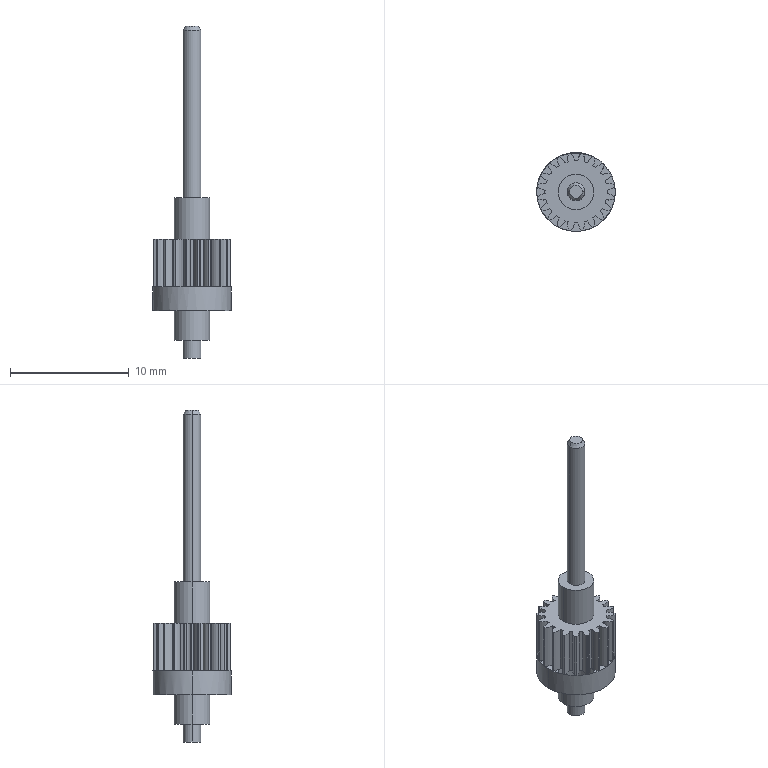Part | SolidWorks | features ICE 5, Extrusion 1, RefAxis 1, RevCut 1 | 1 solid | 105 faces | box 6.634 x 6.634 x 28 mm | volume 248.912 mm3 | cylinder 95 | plane 8 | cone 2 | commonest cylinder face diameters 2.4 x44 5.248 x21 6.6 x20 1.5 x4 3 x4 6.634 x2